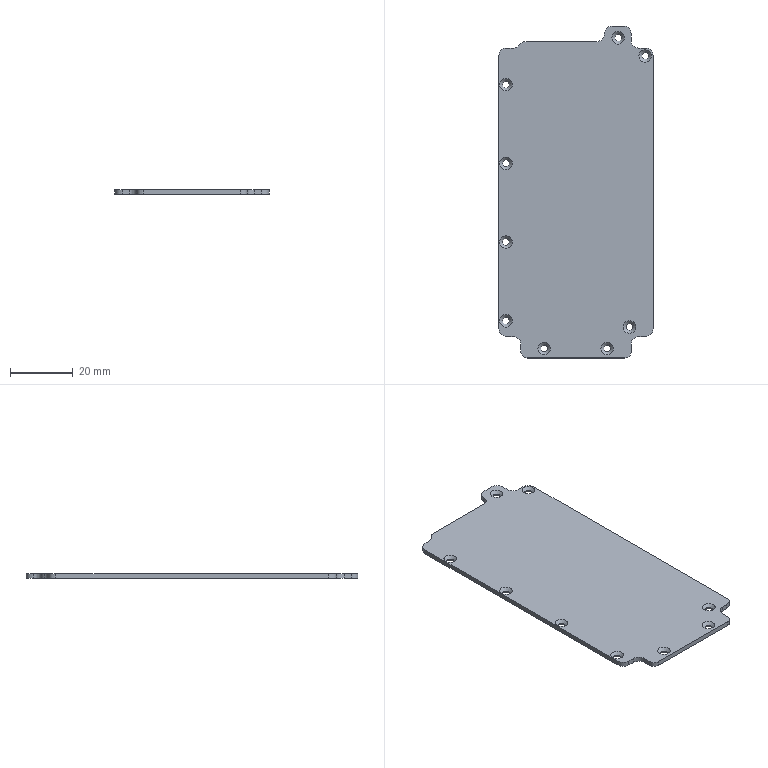Part | STEP file | Final stage cover 2 | 1 solid | 55 faces | box 49 x 105.5 x 1.5 mm | volume 7174 mm3 | cylinder 23 | cone 18 | plane 14 | commonest cylinder face diameters 5 x11 2.2 x9 4 x3